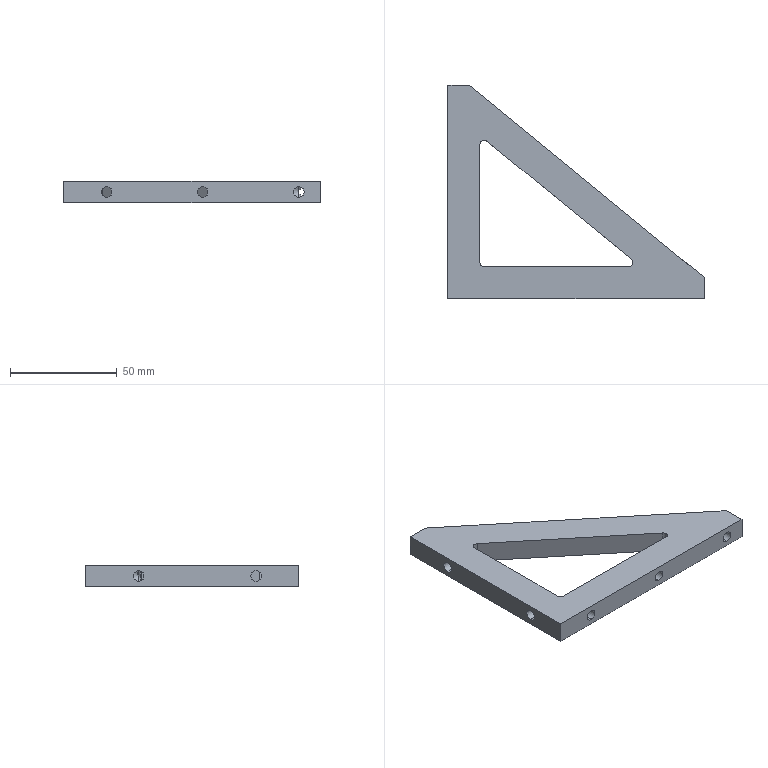Part | STEP file | reinforcing plate 4 | 1 solid | 28 faces | box 120 x 100 x 10 mm | volume 45919 mm3 | cylinder 13 | plane 10 | cone 5 | commonest cylinder face diameters 5 x10 4 x3